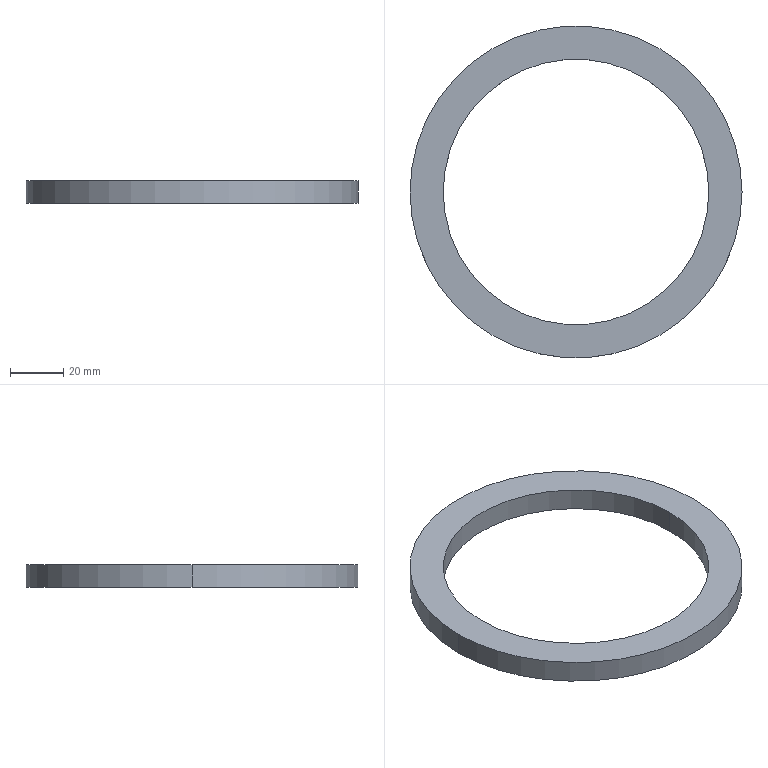Part | SolidWorks | features BaseBody 1 | 1 solid | 6 faces | box 125 x 125 x 8.6 mm | volume 37994 mm3 | cylinder 4 | plane 2 | commonest cylinder face diameters 100 x2 125 x2
STEP:
#1=CARTESIAN_POINT('',(-64.81,49.871,8.6));
#2=VERTEX_POINT('',#1);
#3=CARTESIAN_POINT('',(-164.81,49.871,8.6));
#4=VERTEX_POINT('',#3);
#5=CARTESIAN_POINT('',(-114.81,49.871,8.6));
#6=DIRECTION('',(0.,0.,-1.));
#7=DIRECTION('',(-1.,0.,0.));
#8=AXIS2_PLACEMENT_3D('',#5,#6,#7);
#9=CIRCLE('',#8,50.);
#10=EDGE_CURVE('',#2,#4,#9,.T.);
#11=ORIENTED_EDGE('',*,*,#10,.F.);
#12=CARTESIAN_POINT('',(-64.81,49.871,0.));
#13=VERTEX_POINT('',#12);
#14=CARTESIAN_POINT('',(-64.81,49.871,8.6));
#15=DIRECTION('',(0.,0.,-1.));
#16=VECTOR('',#15,1000.);
#17=LINE('',#14,#16);
#18=EDGE_CURVE('',#2,#13,#17,.T.);
#19=ORIENTED_EDGE('',*,*,#18,.T.);
#20=CARTESIAN_POINT('',(-164.81,49.871,0.));
#21=VERTEX_POINT('',#20);
#22=CARTESIAN_POINT('',(-114.81,49.871,0.));
#23=DIRECTION('',(0.,0.,1.));
#24=DIRECTION('',(-1.,0.,0.));
#25=AXIS2_PLACEMENT_3D('',#22,#23,#24);
#26=CIRCLE('',#25,50.);
#27=EDGE_CURVE('',#21,#13,#26,.T.);
#28=ORIENTED_EDGE('',*,*,#27,.F.);
#29=CARTESIAN_POINT('',(-164.81,49.871,8.6));
#30=DIRECTION('',(0.,0.,-1.));
#31=VECTOR('',#30,1000.);
#32=LINE('',#29,#31);
#33=EDGE_CURVE('',#4,#21,#32,.T.);
#34=ORIENTED_EDGE('',*,*,#33,.F.);
#35=EDGE_LOOP('',(#11,#19,#28,#34));
#36=FACE_OUTER_BOUND('',#35,.T.);
#37=CARTESIAN_POINT('',(-114.81,49.871,8.6));
#38=DIRECTION('',(0.,0.,-1.));
#39=DIRECTION('',(-1.,0.,0.));
#40=AXIS2_PLACEMENT_3D('',#37,#38,#39);
#41=CYLINDRICAL_SURFACE('',#40,50.);
#42=ADVANCED_FACE('',(#36),#41,.F.);
#43=CARTESIAN_POINT('',(-52.31,49.871,8.6));
#44=VERTEX_POINT('',#43);
#45=CARTESIAN_POINT('',(-177.31,49.871,8.6));
#46=VERTEX_POINT('',#45);
#47=CARTESIAN_POINT('',(-114.81,49.871,8.6));
#48=DIRECTION('',(0.,0.,1.));
#49=DIRECTION('',(-1.,0.,0.));
#50=AXIS2_PLACEMENT_3D('',#47,#48,#49);
#51=CIRCLE('',#50,62.5);
#52=EDGE_CURVE('',#44,#46,#51,.T.);
#53=ORIENTED_EDGE('',*,*,#52,.F.);
#54=CARTESIAN_POINT('',(-52.31,49.871,0.));
#55=VERTEX_POINT('',#54);
#56=CARTESIAN_POINT('',(-52.31,49.871,8.6));
#57=DIRECTION('',(0.,0.,-1.));
#58=VECTOR('',#57,1000.);
#59=LINE('',#56,#58);
#60=EDGE_CURVE('',#44,#55,#59,.T.);
#61=ORIENTED_EDGE('',*,*,#60,.T.);
#62=CARTESIAN_POINT('',(-177.31,49.871,0.));
#63=VERTEX_POINT('',#62);
#64=CARTESIAN_POINT('',(-114.81,49.871,0.));
#65=DIRECTION('',(0.,0.,1.));
#66=DIRECTION('',(-1.,0.,0.));
#67=AXIS2_PLACEMENT_3D('',#64,#65,#66);
#68=CIRCLE('',#67,62.5);
#69=EDGE_CURVE('',#55,#63,#68,.T.);
#70=ORIENTED_EDGE('',*,*,#69,.T.);
#71=CARTESIAN_POINT('',(-177.31,49.871,8.6));
#72=DIRECTION('',(0.,0.,-1.));
#73=VECTOR('',#72,1000.);
#74=LINE('',#71,#73);
#75=EDGE_CURVE('',#46,#63,#74,.T.);
#76=ORIENTED_EDGE('',*,*,#75,.F.);
#77=EDGE_LOOP('',(#53,#61,#70,#76));
#78=FACE_OUTER_BOUND('',#77,.T.);
#79=CARTESIAN_POINT('',(-114.81,49.871,8.6));
#80=DIRECTION('',(0.,0.,-1.));
#81=DIRECTION('',(-1.,0.,0.));
#82=AXIS2_PLACEMENT_3D('',#79,#80,#81);
#83=CYLINDRICAL_SURFACE('',#82,62.5);
#84=ADVANCED_FACE('',(#78),#83,.T.);
#85=CARTESIAN_POINT('',(-114.81,49.871,8.6));
#86=DIRECTION('',(0.,0.,-1.));
#87=DIRECTION('',(-1.,0.,0.));
#88=AXIS2_PLACEMENT_3D('',#85,#86,#87);
#89=CIRCLE('',#88,50.);
#90=EDGE_CURVE('',#4,#2,#89,.T.);
#91=ORIENTED_EDGE('',*,*,#90,.T.);
#92=ORIENTED_EDGE('',*,*,#10,.T.);
#93=EDGE_LOOP('',(#91,#92));
#94=FACE_BOUND('',#93,.T.);
#95=CARTESIAN_POINT('',(-114.81,49.871,8.6));
#96=DIRECTION('',(0.,0.,1.));
#97=DIRECTION('',(-1.,0.,0.));
#98=AXIS2_PLACEMENT_3D('',#95,#96,#97);
#99=CIRCLE('',#98,62.5);
#100=EDGE_CURVE('',#46,#44,#99,.T.);
#101=ORIENTED_EDGE('',*,*,#100,.T.);
#102=ORIENTED_EDGE('',*,*,#52,.T.);
#103=EDGE_LOOP('',(#101,#102));
#104=FACE_OUTER_BOUND('',#103,.T.);
#105=CARTESIAN_POINT('',(-114.81,49.871,8.6));
#106=DIRECTION('',(0.,0.,1.));
#107=DIRECTION('',(1.,0.,0.));
#108=AXIS2_PLACEMENT_3D('',#105,#106,#107);
#109=PLANE('',#108);
#110=ADVANCED_FACE('',(#94,#104),#109,.T.);
#111=ORIENTED_EDGE('',*,*,#18,.F.);
#112=ORIENTED_EDGE('',*,*,#90,.F.);
#113=ORIENTED_EDGE('',*,*,#33,.T.);
#114=CARTESIAN_POINT('',(-114.81,49.871,0.));
#115=DIRECTION('',(0.,0.,1.));
#116=DIRECTION('',(-1.,0.,0.));
#117=AXIS2_PLACEMENT_3D('',#114,#115,#116);
#118=CIRCLE('',#117,50.);
#119=EDGE_CURVE('',#13,#21,#118,.T.);
#120=ORIENTED_EDGE('',*,*,#119,.F.);
#121=EDGE_LOOP('',(#111,#112,#113,#120));
#122=FACE_OUTER_BOUND('',#121,.T.);
#123=CARTESIAN_POINT('',(-114.81,49.871,8.6));
#124=DIRECTION('',(0.,0.,-1.));
#125=DIRECTION('',(-1.,0.,0.));
#126=AXIS2_PLACEMENT_3D('',#123,#124,#125);
#127=CYLINDRICAL_SURFACE('',#126,50.);
#128=ADVANCED_FACE('',(#122),#127,.F.);
#129=ORIENTED_EDGE('',*,*,#60,.F.);
#130=ORIENTED_EDGE('',*,*,#100,.F.);
#131=ORIENTED_EDGE('',*,*,#75,.T.);
#132=CARTESIAN_POINT('',(-114.81,49.871,0.));
#133=DIRECTION('',(0.,0.,1.));
#134=DIRECTION('',(-1.,0.,0.));
#135=AXIS2_PLACEMENT_3D('',#132,#133,#134);
#136=CIRCLE('',#135,62.5);
#137=EDGE_CURVE('',#63,#55,#136,.T.);
#138=ORIENTED_EDGE('',*,*,#137,.T.);
#139=EDGE_LOOP('',(#129,#130,#131,#138));
#140=FACE_OUTER_BOUND('',#139,.T.);
#141=CARTESIAN_POINT('',(-114.81,49.871,8.6));
#142=DIRECTION('',(0.,0.,-1.));
#143=DIRECTION('',(-1.,0.,0.));
#144=AXIS2_PLACEMENT_3D('',#141,#142,#143);
#145=CYLINDRICAL_SURFACE('',#144,62.5);
#146=ADVANCED_FACE('',(#140),#145,.T.);
#147=ORIENTED_EDGE('',*,*,#27,.T.);
#148=ORIENTED_EDGE('',*,*,#119,.T.);
#149=EDGE_LOOP('',(#147,#148));
#150=FACE_BOUND('',#149,.T.);
#151=ORIENTED_EDGE('',*,*,#137,.F.);
#152=ORIENTED_EDGE('',*,*,#69,.F.);
#153=EDGE_LOOP('',(#151,#152));
#154=FACE_OUTER_BOUND('',#153,.T.);
#155=CARTESIAN_POINT('',(-114.81,49.871,0.));
#156=DIRECTION('',(0.,0.,1.));
#157=DIRECTION('',(1.,0.,0.));
#158=AXIS2_PLACEMENT_3D('',#155,#156,#157);
#159=PLANE('',#158);
#160=ADVANCED_FACE('',(#150,#154),#159,.F.);
#161=CLOSED_SHELL('',(#42,#84,#110,#128,#146,#160));
#162=MANIFOLD_SOLID_BREP('',#161);
#163=CARTESIAN_POINT('',(0.,0.,0.));
#164=DIRECTION('',(0.,0.,1.));
#165=DIRECTION('',(1.,0.,0.));
#166=AXIS2_PLACEMENT_3D('',#163,#164,#165);
#167=(LENGTH_UNIT()NAMED_UNIT(*)SI_UNIT(.MILLI.,.METRE.));
#168=UNCERTAINTY_MEASURE_WITH_UNIT(LENGTH_MEASURE(0.00001),#167,'','');
#169=(NAMED_UNIT(*)PLANE_ANGLE_UNIT()SI_UNIT($,.RADIAN.));
#170=(NAMED_UNIT(*)SI_UNIT($,.STERADIAN.)SOLID_ANGLE_UNIT());
#171=(GEOMETRIC_REPRESENTATION_CONTEXT(3)GLOBAL_UNCERTAINTY_ASSIGNED_CONTEXT((#168))GLOBAL_UNIT_ASSIGNED_CONTEXT((#167,#169,#170))REPRESENTATION_CONTEXT('',''));
#172=ADVANCED_BREP_SHAPE_REPRESENTATION('',(#162,#166),#171);